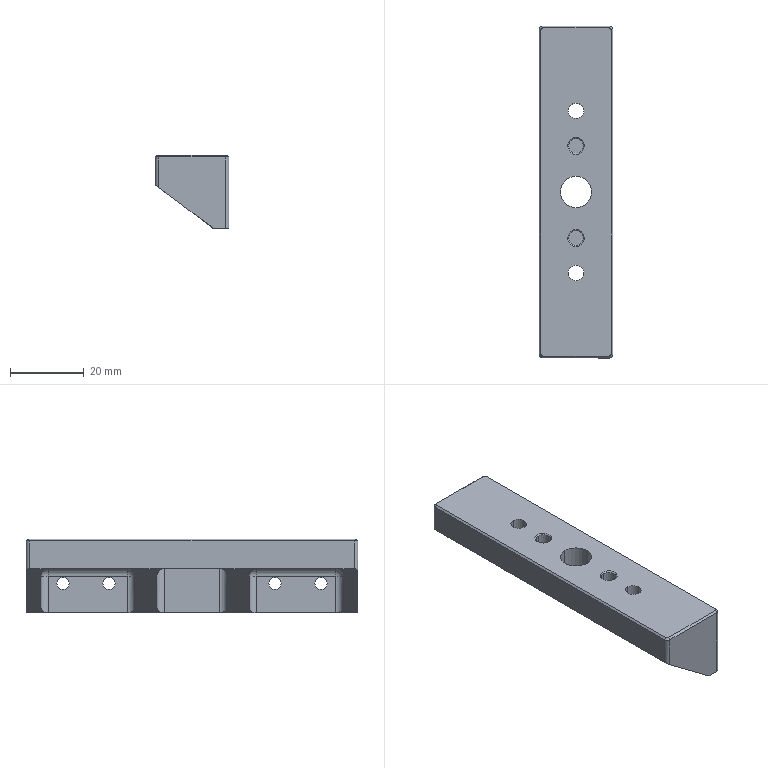NC program | NX | posted with a generic post | part box 20 x 90 x 20 mm
Lines 1 to 986 of 22268:
N10 G17 G21 G94 G90
(FLOOR_WALL_COPY , TOOL : D80)
N12 T19 M6
N14 G54
N16 G17 G0 G90 X-90. Y0. B0. C0. S6500 M3
N18 G43 Z30. H19
N20 Z7.
N22 G94 G1 Z4. F1500.
N24 X-85.
N26 X85.
N28 X90.
N30 Z7.
N32 G0 Z30.
N34 X-90.
N36 Z6.
N38 G1 Z3.
N40 X-85.
N42 X85.
N44 X90.
N46 Z6.
N48 G0 Z30.
N50 X-90.
N52 Z5.
N54 G1 Z2.
N56 X-85.
N58 X85.
N60 X90.
N62 Z5.
N64 G0 Z30.
N66 X-90.
N68 Z4.
N70 G1 Z1.
N72 X-85.
N74 X85.
N76 X90.
N78 Z4.
N80 G0 Z30.
N82 X-90.
N84 Z3.
N86 G1 Z0.
N88 X-85.
N90 X85.
N92 X90.
N94 Z3.
N96 G0 Z30.
N98 M5
(CAVITY_MILL , TOOL : D10)
N100 T15 M6
N102 G54
N104 G17 G0 G90 X-8.081 Y-16.996 B0. C0. S9500 M3
N106 G43 Z30. H15
N108 Z0.508
N110 G94 G1 Z-0.992 F1000.
N112 X-11.545 Y-10.996
N114 G3 X-12.411 Y-10.496 R1.
N116 G1 Y-5.996
N118 X-4.377 F3000.
N120 G2 X-2.441 Y-5.559 R4.5
N122 G1 X2.621 Y-5.56
N124 G2 X4.552 Y-5.996 R4.5
N126 G1 X20.578
N128 G2 X22.734 Y-5.541 R4.5
N130 G1 X23.214 Y-5.56
N132 X34.119
N134 G2 X36.052 Y-5.996 R4.5
N136 G1 X40.559
N138 Y-4.981
N140 G2 X35.921 Y-3.6 R9.806
N142 G1 X20.601
N144 G2 X15.634 Y-4.989 R10.196
N146 G1 X9.4
N148 G2 X4.42 Y-3.6 R9.73
N150 G1 X-4.431
N152 G2 X-9.404 Y-4.989 R9.73
N154 G1 X-15.645
N156 G2 X-20.601 Y-3.6 R10.226
N158 G1 X-35.924
N160 G2 X-40.559 Y-4.982 R9.72
N162 G1 Y-5.996
N164 X-35.876
N166 G2 X-33.941 Y-5.559 R4.5
N168 G1 X-22.377 Y-5.56
N170 G2 X-20.445 Y-5.996 R4.5
N172 G1 X-12.411
N174 Y-10.496
N176 X-2.465
N178 X-2.443 Y-10.184
N180 X-2.442 Y-10.059
N182 X2.619 Y-10.06
N184 G3 X2.654 Y-10.496 R5.476
N186 G1 X22.534
N188 X22.557 Y-10.038
N190 X23.126 Y-10.06
N192 X34.119
N194 G3 X34.154 Y-10.496 R5.269
N196 G1 X45.004
N198 X45.059 Y-10.493
N200 Y-0.488
N202 X40.909 Y-0.489
N204 G2 X37.372 Y0.9 R5.306
N206 G1 X19.19
N208 G2 X15.585 Y-0.489 R5.696
N210 G1 X9.409
N212 G2 X5.88 Y0.9 R5.23
N214 G1 X-5.891
N216 G2 X-9.415 Y-0.489 R5.23
N218 G1 X-15.591
N220 G2 X-19.193 Y0.9 R5.726
N222 G1 X-37.386
N224 G2 X-40.915 Y-0.489 R5.22
N226 G1 X-45.059 Y-0.488
N228 Y-1.888
N230 Y-10.493
N232 X-45.004 Y-10.496
N234 X-33.965
N236 X-33.943 Y-10.167
N238 X-33.941 Y-10.059
N240 X-22.378 Y-10.06
N242 X-22.345 Y-10.496
N244 X-12.411
N246 G2 X-11.545 Y-10.996 R1.
N248 G1 X-8.081 Y-16.996
N250 Z0.508
N252 G0 X-14.854 Z-0.483
N254 G1 Z-1.983 F1000.
N256 X-18.318 Y-10.996
N258 G3 X-19.184 Y-10.496 R1.
N260 G1 Y-5.996
N262 X-17.923 F3000.
N264 G2 X-22.174 Y-3.6 R9.614
N266 G1 X-34.345
N268 G2 X-38.549 Y-5.996 R9.442
N270 G1 X-35.876
N272 G2 X-33.941 Y-5.559 R4.5
N274 G1 X-22.377 Y-5.56
N276 G2 X-20.445 Y-5.996 R4.5
N278 G1 X-19.184
N280 Y-10.496
N282 X-7.071
N284 Y-5.996
N286 X-4.378
N288 G2 X-2.441 Y-5.559 R4.5
N290 G1 X2.621 Y-5.56
N292 G2 X4.552 Y-5.996 R4.5
N294 G1 X7.068
N296 G2 X2.827 Y-3.6 R9.58
N298 G1 X-2.828
N300 G2 X-7.071 Y-5.996 R9.584
N302 G1 Y-10.496
N304 X-2.465
N306 X-2.443 Y-10.184
N308 X-2.442 Y-10.059
N310 X2.619 Y-10.06
N312 G3 X2.654 Y-10.496 R5.476
N314 G1 X17.923
N316 Y-5.996
N318 X20.578
N320 G2 X22.734 Y-5.541 R4.5
N322 G1 X23.214 Y-5.56
N324 X34.119
N326 G2 X36.052 Y-5.996 R4.5
N328 G1 X38.549
N330 G2 X34.345 Y-3.6 R9.442
N332 G1 X22.174
N334 G2 X17.923 Y-5.996 R9.613
N336 G1 Y-10.496
N338 X22.534
N340 X22.557 Y-10.038
N342 X23.126 Y-10.06
N344 X34.119
N346 G3 X34.154 Y-10.496 R5.269
N348 G1 X45.004
N350 X45.059 Y-10.493
N352 Y-1.81
N354 X40.967 Y-1.811
N356 G2 X37.472 Y-0.363 R4.942
N358 X36.43 Y0.9 R8.564
N360 G1 X19.997
N362 G2 X15.5 Y-1.811 R5.113
N364 G1 X9.5
N366 G2 X5.011 Y0.9 R5.08
N368 G1 X-5.011
N370 G2 X-9.5 Y-1.811 R5.084
N372 G1 X-15.5
N374 G2 X-19.997 Y0.9 R5.114
N376 G1 X-36.43
N378 G2 X-37.472 Y-0.363 R8.564
N380 X-40.967 Y-1.811 R4.942
N382 G1 X-45.059 Y-1.81
N384 Y-3.211
N386 Y-10.493
N388 X-45.004 Y-10.496
N390 X-33.965
N392 X-33.943 Y-10.167
N394 X-33.941 Y-10.059
N396 X-22.378 Y-10.06
N398 X-22.345 Y-10.496
N400 X-19.184
N402 G2 X-18.318 Y-10.996 R1.
N404 G1 X-14.854 Y-16.996
N406 Z-0.483
N408 G0 X-17.797 Z-1.475
N410 G1 Z-2.975 F1000.
N412 X-21.512 Y-10.56
N414 G3 X-22.378 Y-10.06 R1.
N416 G1 X-22.377 Y-5.56
N418 G2 X-21.26 Y-5.701 R4.5 F3000.
N420 X-23.306 Y-3.6 R9.607
N422 G1 X-33.193
N424 G2 X-35.355 Y-5.787 R9.605
N426 X-33.941 Y-5.559 R4.5
N428 G1 X-22.377 Y-5.56
N430 X-22.378 Y-10.06
N432 X-22.345 Y-10.496
N434 X-2.465
N436 X-2.443 Y-10.184
N438 X-2.442 Y-10.059
N440 X-3.852 Y-5.785
N442 G2 X-2.441 Y-5.559 R4.5
N444 G1 X2.621 Y-5.56
N446 G2 X3.74 Y-5.702 R4.5
N448 X1.693 Y-3.6 R9.606
N450 G1 X-1.693
N452 G2 X-3.852 Y-5.785 R9.602
N454 G1 X-2.442 Y-10.059
N456 X2.619 Y-10.06
N458 G3 X2.654 Y-10.496 R5.476
N460 G1 X22.534
N462 X22.557 Y-10.038
N464 X21.195 Y-5.749
N466 G2 X22.734 Y-5.541 R4.5
N468 G1 X23.214 Y-5.56
N470 X34.119
N472 G2 X35.24 Y-5.702 R4.5
N474 X33.194 Y-3.6 R9.602
N476 G1 X23.305
N478 G2 X21.195 Y-5.749 R9.608
N480 G1 X22.557 Y-10.038
N482 X23.126 Y-10.06
N484 X34.119
N486 G3 X34.154 Y-10.496 R5.269
N488 G1 X45.004
N490 X45.059 Y-10.493
N492 Y-3.133
N494 X41.
N496 G2 X36.027 Y0.9 R5.102
N498 G1 X20.474
N500 G2 X15.5 Y-3.133 R5.108
N502 G1 X9.5
N504 G2 X4.525 Y0.9 R5.106
N506 G1 X-4.527
N508 G2 X-9.5 Y-3.133 R5.102
N510 G1 X-15.5
N512 G2 X-20.474 Y0.9 R5.107
N514 G1 X-36.026
N516 G2 X-41. Y-3.133 R5.105
N518 G1 X-45.059
N520 Y-10.493
N522 X-45.004 Y-10.496
N524 X-33.965
N526 X-33.943 Y-10.167
N528 X-33.941 Y-10.059
N530 X-22.378 Y-10.06
N532 G2 X-21.512 Y-10.56 R1.
N534 G1 X-17.797 Y-16.996
N536 Z-1.475
N538 G0 X-23.669 Y-16.997 Z-2.467
N540 G1 Z-3.967 F1000.
N542 X-27.384 Y-10.56
N544 G3 X-28.25 Y-10.06 R1.
N546 G1 Y-5.56
N548 X-22.808 F3000.
N550 G2 X-24.098 Y-3.6 R9.633
N552 G1 X-32.402
N554 G2 X-33.692 Y-5.559 R9.635
N556 G1 X-28.25 Y-5.56
N558 Y-10.06
N560 X-22.378
N562 X-22.345 Y-10.497
N564 X-2.465
N566 X-2.443 Y-10.184
N568 X-2.442 Y-10.059
N570 X-2.21
N572 X-2.208 Y-5.559
N574 X2.209 Y-5.56
N576 G2 X0.914 Y-3.6 R9.666
N578 G1 X-0.914
N580 G2 X-2.208 Y-5.559 R9.666
N582 G1 X-2.21 Y-10.059
N584 X2.619 Y-10.06
N586 G3 X2.654 Y-10.497 R5.476
N588 G1 X22.534
N590 X22.557 Y-10.038
N592 X22.644 Y-10.041
N594 X22.821 Y-5.545
N596 X23.214 Y-5.56
N598 X33.693
N600 G2 X32.402 Y-3.6 R9.635
N602 G1 X24.098
N604 G2 X22.821 Y-5.545 R9.634
N606 G1 X22.644 Y-10.041
N608 X23.126 Y-10.06
N610 X34.119
N612 G3 X34.154 Y-10.497 R5.269
N614 G1 X45.003
N616 X45.059 Y-10.493
N618 Y-4.455
N620 X41. Y-4.456
N622 G2 X35.904 Y0.475 R5.135
N624 X35.9 Y0.782 R5.136
N626 G1 X35.904 Y0.9
N628 X20.6
N630 Y0.712
N632 G2 X15.5 Y-4.456 R5.134
N634 G1 X9.476 Y-4.455
N636 G2 X4.508 Y-0.339 R5.166
N638 X4.4 Y0.756 R5.166
N640 G1 X4.401 Y0.9
N642 X-4.4
N644 Y0.711
N646 G2 X-9.5 Y-4.456 R5.166
N648 G1 X-15.5
N650 G2 X-20.546 Y-0.068 R5.133
N652 X-20.6 Y0.746 R5.134
N654 G1 X-20.597 Y0.9
N656 X-35.9
N658 Y0.711
N660 G2 X-41. Y-4.456 R5.135
N662 G1 X-45.059 Y-4.455
N664 Y-10.493
N666 X-45.003 Y-10.497
N668 X-33.965
N670 X-33.943 Y-10.167
N672 X-33.941 Y-10.059
N674 X-28.25 Y-10.06
N676 G2 X-27.384 Y-10.56 R1.
N678 G1 X-23.669 Y-16.997
N680 Z-2.467
N682 G0 X-23.671 Z-3.458
N684 G1 Z-4.958 F1000.
N686 X-27.387 Y-10.56
N688 G3 X-28.253 Y-10.06 R1.
N690 G1 Y-5.56
N692 X-23.752 F3000.
N694 G2 X-24.636 Y-3.6 R9.633
N696 G1 X-31.868
N698 G2 X-32.754 Y-5.559 R9.647
N700 G1 X-28.253 Y-5.56
N702 Y-10.06
N704 X-22.378
N706 X-22.345 Y-10.497
N708 X-2.465
N710 X-2.443 Y-10.184
N712 X-2.442 Y-10.059
N714 X-1.268
N716 X-1.267 Y-5.559
N718 X1.267 Y-5.56
N720 G2 X0.377 Y-3.6 R9.678
N722 G1 X-0.377
N724 G2 X-1.267 Y-5.559 R9.678
N726 G1 X-1.268 Y-10.059
N728 X2.619 Y-10.06
N730 G3 X2.654 Y-10.497 R5.476
N732 G1 X22.534
N734 X22.557 Y-10.038
N736 X23.126 Y-10.06
N738 X23.752
N740 Y-5.56
N742 X32.754
N744 G2 X31.868 Y-3.6 R9.647
N746 G1 X24.636
N748 G2 X23.752 Y-5.56 R9.633
N750 G1 Y-10.06
N752 X34.119
N754 G3 X34.154 Y-10.497 R5.269
N756 G1 X45.003
N758 X45.059 Y-10.494
N760 Y-5.777
N762 X41. Y-5.778
N764 G2 X35.9 Y-0.611 R5.147
N766 G1 Y-0.5
N768 Y0.782
N770 X35.903 Y0.9
N772 X20.6
N774 Y-0.611
N776 G2 X15.5 Y-5.778 R5.133
N778 G1 X9.5
N780 G2 X4.4 Y-0.611 R5.178
N782 G1 Y0.9
N784 X-4.4
N786 Y-0.611
N788 G2 X-9.5 Y-5.778 R5.178
N790 G1 X-15.5
N792 G2 X-20.6 Y-0.611 R5.133
N794 G1 Y0.746
N796 X-20.597 Y0.9
N798 X-35.9
N800 Y-0.611
N802 G2 X-41. Y-5.778 R5.147
N804 G1 X-45.059 Y-5.777
N806 Y-10.494
N808 X-45.003 Y-10.497
N810 X-33.965
N812 X-33.943 Y-10.167
N814 X-33.941 Y-10.059
N816 X-28.253 Y-10.06
N818 G2 X-27.387 Y-10.56 R1.
N820 G1 X-23.671 Y-16.997
N822 Z-3.458
N824 G0 X-23.668 Z-4.45
N826 G1 Z-5.95 F1000.
N828 X-27.384 Y-10.56
N830 G3 X-28.25 Y-10.06 R1.
N832 G1 Y-5.56
N834 X-24.405 F3000.
N836 G2 X-24.961 Y-3.6 R9.633
N838 G1 X-31.539
N840 G2 X-32.095 Y-5.559 R9.633
N842 G1 X-28.25 Y-5.56
N844 Y-10.06
N846 X-22.378
N848 X-22.345 Y-10.497
N850 X-2.465
N852 X-2.443 Y-10.184
N854 X-2.442 Y-10.059
N856 X-0.596
N858 X-0.595 Y-5.559
N860 X0.595
N862 G2 X0.039 Y-3.6 R9.633
N864 G1 X-0.039
N866 G2 X-0.595 Y-5.559 R9.633
N868 G1 X-0.596 Y-10.059
N870 X2.619 Y-10.06
N872 G3 X2.654 Y-10.497 R5.476
N874 G1 X22.534
N876 X22.557 Y-10.038
N878 X23.126 Y-10.06
N880 X24.405
N882 Y-5.56
N884 X32.095
N886 G2 X31.539 Y-3.6 R9.633
N888 G1 X24.961
N890 G2 X24.405 Y-5.56 R9.633
N892 G1 Y-10.06
N894 X34.119
N896 G3 X34.154 Y-10.497 R5.269
N898 G1 X45.003
N900 X45.059 Y-10.494
N902 Y-7.099
N904 X41. Y-7.1
N906 G2 X35.9 Y-1.933 R5.133
N908 G1 Y0.782
N910 X35.903 Y0.9
N912 X20.6
N914 Y-1.933
N916 G2 X15.5 Y-7.1 R5.133
N918 G1 X9.475
N920 G2 X4.4 Y-1.933 R5.133
N922 G1 Y0.9
N924 X-4.4
N926 Y-1.933
N928 G2 X-9.5 Y-7.1 R5.133
N930 G1 X-15.5
N932 G2 X-20.6 Y-1.933 R5.133
N934 G1 Y0.746
N936 X-20.598 Y0.9
N938 X-35.9
N940 Y-1.933
N942 G2 X-41. Y-7.1 R5.133
N944 G1 X-45.059 Y-7.099
N946 Y-10.494
N948 X-45.003 Y-10.497
N950 X-33.965
N952 X-33.943 Y-10.167
N954 X-33.941 Y-10.059
N956 X-28.25 Y-10.06
N958 G2 X-27.384 Y-10.56 R1.
N960 G1 X-23.668 Y-16.997
N962 Z-4.45
N964 G0 Z-5.442
N966 G1 Z-6.942 F1000.
N968 X-27.384 Y-10.56
N970 G3 X-28.25 Y-10.06 R1.
N972 G1 Y-5.56
N974 X-24.829 F3000.
N976 G2 X-25.095 Y-3.6 R9.633
N978 G1 X-31.405
N980 G2 X-31.671 Y-5.559 R9.633
N982 G1 X-28.25 Y-5.56
N984 Y-10.06
N986 X-22.378
N988 X-22.345 Y-10.497
N990 X-2.465
N992 X-2.443 Y-10.184
N994 X-2.442 Y-10.059
N996 X-0.172
N998 X-0.171 Y-5.559
N1000 X0.171
N1002 G2 X0. Y-4.674 R9.633
N1004 X-0.171 Y-5.559 R9.633
N1006 G1 X-0.172 Y-10.059
N1008 X2.619 Y-10.06
N1010 G3 X2.654 Y-10.497 R5.476
N1012 G1 X22.534
N1014 X22.557 Y-10.038
N1016 X23.126 Y-10.06
N1018 X24.829
N1020 Y-5.56
N1022 X31.671
N1024 G2 X31.405 Y-3.6 R9.633
N1026 G1 X25.095
N1028 G2 X24.829 Y-5.56 R9.633
N1030 G1 Y-10.06
N1032 X34.119
N1034 G3 X34.154 Y-10.497 R5.269
N1036 G1 X45.003
N1038 X45.059 Y-10.494
N1040 Y-8.421
N1042 X41. Y-8.422
N1044 G2 X35.9 Y-3.256 R5.133
N1046 G1 Y0.782
N1048 X35.902 Y0.9
N1050 X20.6
N1052 Y-3.256
N1054 G2 X15.5 Y-8.422 R5.133
N1056 G1 X9.5
N1058 G2 X4.4 Y-3.256 R5.133
N1060 G1 Y0.9
N1062 X-4.4
N1064 Y-3.256
N1066 G2 X-9.5 Y-8.422 R5.133
N1068 G1 X-15.5
N1070 G2 X-20.6 Y-3.256 R5.133
N1072 G1 Y0.746
N1074 X-20.598 Y0.9
N1076 X-35.9
N1078 Y-3.256
N1080 G2 X-41. Y-8.422 R5.133
N1082 G1 X-45.059 Y-8.421
N1084 Y-10.494
N1086 X-45.003 Y-10.497
N1088 X-33.965
N1090 X-33.943 Y-10.167
N1092 X-33.941 Y-10.059
N1094 X-28.25 Y-10.06
N1096 G2 X-27.384 Y-10.56 R1.
N1098 G1 X-23.668 Y-16.997
N1100 Z-5.442
N1102 G0 Z-6.433
N1104 G1 Z-7.933 F1000.
N1106 X-27.385 Y-10.56
N1108 G3 X-28.251 Y-10.06 R1.
N1110 G1 X-28.25 Y-5.56
N1112 X-25.053 F3000.
N1114 G2 X-25.1 Y-4.567 R9.639
N1116 G1 Y-3.6
N1118 X-31.4
N1120 Y-4.569
N1122 G2 X-31.448 Y-5.559 R9.643
N1124 G1 X-28.25 Y-5.56
N1126 X-28.251 Y-10.06
N1128 X-22.378
N1130 X-22.345 Y-10.497
N1132 X-18.298
N1134 G3 X-15.5 Y-11.144 R6.539
N1136 G1 X-9.478
N1138 G3 X-6.733 Y-10.497 R6.58
N1140 G1 X-2.465
N1142 X-2.443 Y-10.184
N1144 X-2.442 Y-10.059
N1146 X2.619 Y-10.06
N1148 G3 X2.654 Y-10.497 R5.476
N1150 G1 X6.733
N1152 G3 X9.5 Y-11.144 R6.58
N1154 G1 X15.511
N1156 G3 X18.298 Y-10.497 R6.539
N1158 G1 X22.534
N1160 X22.557 Y-10.038
N1162 X23.126 Y-10.06
N1164 X25.053
N1166 Y-5.56
N1168 X31.448
N1170 G2 X31.4 Y-4.569 R9.643
N1172 G1 Y-3.6
N1174 X25.1
N1176 Y-4.567
N1178 G2 X25.053 Y-5.56 R9.639
N1180 G1 Y-10.06
N1182 X34.119
N1184 G3 X34.154 Y-10.497 R5.269
N1186 G1 X38.205
N1188 G3 X41. Y-11.144 R6.543
N1190 G1 X45.059
N1192 Y-9.743
N1194 X41. Y-9.744
N1196 G2 X35.9 Y-4.578 R5.143
N1198 G1 Y0.782
N1200 X35.901 Y0.9
N1202 X20.6
N1204 Y-4.578
N1206 G2 X15.5 Y-9.744 R5.139
N1208 G1 X9.5
N1210 G2 X4.4 Y-4.578 R5.18
N1212 G1 Y0.9
N1214 X-4.4
N1216 Y-4.578
N1218 G2 X-9.5 Y-9.744 R5.18
N1220 G1 X-15.529
N1222 G2 X-20.6 Y-4.578 R5.139
N1224 G1 Y0.746
N1226 X-20.599 Y0.9
N1228 X-35.9
N1230 Y-4.578
N1232 G2 X-41. Y-9.744 R5.143
N1234 G1 X-45.059 Y-9.743
N1236 Y-10.494
N1238 Y-11.144
N1240 X-40.988
N1242 G3 X-38.205 Y-10.497 R6.543
N1244 G1 X-33.965
N1246 X-33.943 Y-10.167
N1248 X-33.941 Y-10.059
N1250 X-28.251 Y-10.06
N1252 G2 X-27.385 Y-10.56 R1.
N1254 G1 X-23.668 Y-16.997
N1256 Z-6.433
N1258 G0 Z-7.425
N1260 G1 Z-8.925 F1000.
N1262 X-27.384 Y-10.56
N1264 G3 X-28.25 Y-10.06 R1.
N1266 G1 Y-5.56
N1268 X-25.1 F3000.
N1270 Y-3.6
N1272 X-31.4
N1274 Y-5.559
N1276 X-28.25 Y-5.56
N1278 Y-10.06
N1280 X-22.378
N1282 X-22.345 Y-10.497
N1284 X-20.142
N1286 G3 X-15.5 Y-12.467 R6.533
N1288 G1 X-9.482
N1290 G3 X-4.878 Y-10.497 R6.567
N1292 G1 X-2.465
N1294 X-2.443 Y-10.184
N1296 X-2.442 Y-10.059
N1298 X2.619 Y-10.06
N1300 G3 X2.654 Y-10.497 R5.476
N1302 G1 X4.878
N1304 G3 X9.5 Y-12.467 R6.567
N1306 G1 X15.509
N1308 G3 X20.142 Y-10.497 R6.533
N1310 G1 X22.534
N1312 X22.557 Y-10.038
N1314 X23.126 Y-10.06
N1316 X25.1
N1318 Y-5.56
N1320 X31.4
N1322 Y-3.6
N1324 X25.1
N1326 Y-5.56
N1328 Y-10.06
N1330 X34.119
N1332 G3 X34.154 Y-10.497 R5.269
N1334 G1 X36.365
N1336 G3 X41. Y-12.467 R6.544
N1338 G1 X45.059 Y-12.466
N1340 Y-11.066
N1342 X41. Y-11.067
N1344 G2 X35.9 Y-5.9 R5.144
N1346 G1 Y0.782
N1348 X35.901 Y0.9
N1350 X34.501
N1352 X20.6
N1354 Y-5.9
N1356 G2 X15.5 Y-11.067 R5.133
N1358 G1 X9.5
N1360 G2 X4.4 Y-5.9 R5.167
N1362 G1 Y0.9
N1364 X-4.4
N1366 Y-5.9
N1368 G2 X-9.5 Y-11.067 R5.167
N1370 G1 X-15.5
N1372 G2 X-20.6 Y-5.9 R5.133
N1374 G1 Y0.746
N1376 X-20.599 Y0.9
N1378 X-21.999
N1380 X-35.9
N1382 Y-5.9
N1384 G2 X-41. Y-11.067 R5.144
N1386 G1 X-45.059 Y-11.066
N1388 Y-12.466
N1390 X-40.988 Y-12.467
N1392 G3 X-36.365 Y-10.497 R6.544
N1394 G1 X-33.965
N1396 X-33.943 Y-10.167
N1398 X-33.941 Y-10.059
N1400 X-28.25 Y-10.06
N1402 G2 X-27.384 Y-10.56 R1.
N1404 G1 X-23.668 Y-16.997
N1406 Z-7.425
N1408 G0 Y-16.998 Z-8.417
N1410 G1 Z-9.917 F1000.
N1412 X-27.384 Y-10.56
N1414 G3 X-28.25 Y-10.06 R1.
N1416 G1 Y-5.56
N1418 X-25.1 F3000.
N1420 Y-3.6
N1422 X-31.4
N1424 Y-5.559
N1426 X-28.25 Y-5.56
N1428 Y-10.06
N1430 X-22.378
N1432 X-22.345 Y-10.498
N1434 X-21.134
N1436 G3 X-15.5 Y-13.789 R6.545
N1438 G1 X-9.491
N1440 G3 X-3.861 Y-10.498 R6.533
N1442 G1 X-2.465
N1444 X-2.443 Y-10.184
N1446 X-2.442 Y-10.059
N1448 X2.619 Y-10.06
N1450 G3 X2.654 Y-10.498 R5.476
N1452 G1 X3.862
N1454 G3 X9.5 Y-13.789 R6.535
N1456 G1 X15.509
N1458 G3 X21.139 Y-10.498 R6.533
N1460 G1 X22.534
N1462 X22.557 Y-10.038
N1464 X23.126 Y-10.06
N1466 X25.1
N1468 Y-5.56
N1470 X31.4
N1472 Y-3.6
N1474 X25.1
N1476 Y-5.56
N1478 Y-10.06
N1480 X34.119
N1482 G3 X34.154 Y-10.498 R5.269
N1484 G1 X35.361
N1486 G3 X41. Y-13.789 R6.533
N1488 G1 X45.045
N1490 X45.059 Y-13.586
N1492 Y-12.388
N1494 X41. Y-12.389
N1496 G2 X35.9 Y-7.222 R5.133
N1498 G1 Y-5.56
N1500 Y0.9
N1502 X20.6
N1504 Y-7.222
N1506 G2 X15.5 Y-12.389 R5.133
N1508 G1 X9.474
N1510 G2 X4.4 Y-7.222 R5.135
N1512 G1 Y0.9
N1514 X-4.4
N1516 Y-7.222
N1518 G2 X-9.5 Y-12.389 R5.133
N1520 G1 X-15.5
N1522 G2 X-20.6 Y-7.222 R5.145
N1524 G1 Y0.746
N1526 Y0.9
N1528 X-35.9
N1530 Y-7.222
N1532 G2 X-41. Y-12.389 R5.133
N1534 G1 X-45.059 Y-12.388
N1536 Y-13.585
N1538 X-45.062 Y-13.788
N1540 X-40.991 Y-13.789
N1542 G3 X-35.361 Y-10.498 R6.533
N1544 G1 X-33.965
N1546 X-33.943 Y-10.167
N1548 X-33.941 Y-10.059
N1550 X-28.25 Y-10.06
N1552 G2 X-27.384 Y-10.56 R1.
N1554 G1 X-23.668 Y-16.998
N1556 Z-8.417
N1558 G0 Z-9.408
N1560 G1 Z-10.908 F1000.
N1562 X-27.384 Y-10.56
N1564 G3 X-28.25 Y-10.06 R1.
N1566 G1 Y-5.56
N1568 X-25.331 F3000.
N1570 Y-3.831
N1572 X-31.169
N1574 Y-5.559
N1576 X-28.25 Y-5.56
N1578 Y-10.06
N1580 X-22.378
N1582 X-22.345 Y-10.498
N1584 X-21.962
N1586 G3 X-16.978 Y-14.998 R6.458
N1588 G1 X-8.048
N1590 G3 X-3.045 Y-10.498 R6.487
N1592 G1 X-2.465
N1594 X-2.443 Y-10.184
N1596 X-2.442 Y-10.059
N1598 X2.619 Y-10.06
N1600 G3 X2.654 Y-10.498 R5.476
N1602 G1 X3.045
N1604 G3 X8.048 Y-14.998 R6.486
N1606 G1 X16.952
N1608 G3 X21.955 Y-10.498 R6.487
N1610 G1 X22.534
N1612 X22.557 Y-10.038
N1614 X23.126 Y-10.06
N1616 X25.331
N1618 Y-5.56
N1620 X31.169
N1622 Y-3.831
N1624 X25.331
N1626 Y-5.56
N1628 Y-10.06
N1630 X34.119
N1632 G3 X34.154 Y-10.498 R5.269
N1634 G1 X34.545
N1636 G3 X39.548 Y-14.998 R6.486
N1638 G1 X44.492
N1640 X44.603 Y-14.929
N1642 X44.748 Y-14.809
N1644 X44.976 Y-14.635
N1646 X45.019 Y-14.628
N1648 X44.999 Y-14.589
N1650 X45.006 Y-14.355
N1652 X45.051 Y-13.71
N1654 X40.735 Y-13.711
N1656 G2 X35.669 Y-8.605 R5.086
N1658 G1 Y-0.731
N1660 Y0.669
N1662 X20.831
N1664 Y-0.731
N1666 Y-8.606
N1668 G2 X15.761 Y-13.711 R5.087
N1670 G1 X9.235
N1672 G2 X4.169 Y-8.605 R5.086
N1674 G1 Y0.9
N1676 X-4.169
N1678 Y-8.606
N1680 G2 X-9.239 Y-13.711 R5.087
N1682 G1 X-15.773
N1684 G2 X-20.831 Y-8.653 R5.058
N1686 G1 Y-0.731
N1688 Y0.669
N1690 X-35.669
N1692 Y-0.731
N1694 Y-8.606
N1696 G2 X-40.739 Y-13.711 R5.087
N1698 G1 X-45.061 Y-13.71
N1700 X-45.068 Y-14.251
N1702 X-45.061 Y-14.28
N1704 X-45.007 Y-14.378
N1706 X-44.903 Y-14.606
N1708 X-44.699 Y-14.88
N1710 X-44.674 Y-14.9
N1712 X-44.442 Y-14.998
N1714 X-39.548
N1716 G3 X-34.545 Y-10.498 R6.487
N1718 G1 X-33.965
N1720 X-33.943 Y-10.167
N1722 X-33.941 Y-10.059
N1724 X-28.25 Y-10.06
N1726 G2 X-27.384 Y-10.56 R1.
N1728 G1 X-23.668 Y-16.998
N1730 Z-9.408
N1732 G0 Z-10.4
N1734 G1 Z-11.9 F1000.
N1736 X-27.384 Y-10.56
N1738 G3 X-28.25 Y-10.06 R1.
N1740 G1 Y-5.56
N1742 X-26.831 F3000.
N1744 Y-5.331
N1746 X-29.669
N1748 Y-5.559
N1750 X-28.25 Y-5.56
N1752 Y-10.06
N1754 X-22.378
N1756 X-22.341 Y-10.534
N1758 X-22.196 Y-11.309
N1760 X-21.916 Y-12.086
N1762 X-21.785 Y-12.293
N1764 X-21.701 Y-12.507
N1766 X-21.692 Y-12.563
N1768 X-21.637 Y-12.547
N1770 X-21.613 Y-12.584
N1772 X-21.606 Y-12.656
N1774 X-21.597 Y-12.682
N1776 X-21.53 Y-12.781
N1778 X-21.433 Y-12.862
N1780 X-20.853 Y-13.609
N1782 X-20.242 Y-14.14
N1784 X-20.181 Y-14.167
N1786 G3 X-18.232 Y-14.998 R5.26
N1788 G1 X-17.638
N1790 G2 X-22.331 Y-9.757 R5.211
N1792 G1 Y-0.831
N1794 X-34.169
N1796 Y-9.989
N1798 G2 X-38.753 Y-14.998 R5.096
N1800 G1 X-38.265
N1802 G3 X-36.557 Y-14.403 R6.548
N1804 X-34.111 Y-11.299 R5.676
N1806 G1 X-33.967 Y-10.527
N1808 X-33.965 Y-10.498
N1810 X-33.942 Y-10.131
N1812 X-33.941 Y-10.059
N1814 X-28.25 Y-10.06
N1816 G2 X-27.384 Y-10.56 R1.
N1818 G1 X-23.668 Y-16.998
N1820 Z-10.4
N1822 G0 Z30.
N1824 X-4.497
N1826 Z-10.4
N1828 G1 Z-11.9 F1000.
N1830 X-0.777 Y-10.559
N1832 G2 X0.089 Y-10.059 R1.
N1834 G1 X2.619 Y-10.06 F3000.
N1836 G3 X2.654 Y-10.498 R5.476
N1838 X3.513 Y-12.851 R5.476
N1840 G1 X3.801 Y-13.394
N1842 X3.823 Y-13.417
N1844 X4.172 Y-13.634
N1846 X4.547 Y-13.963
N1848 X4.593 Y-13.988
N1850 G3 X6.838 Y-14.998 R5.931
N1852 G1 X7.362
N1854 G2 X2.669 Y-9.757 R5.211
N1856 G1 Y0.9
N1858 X-2.669
N1860 Y-9.757
N1862 G2 X-7.364 Y-14.998 R5.213
N1864 G1 X-6.806
N1866 G3 X-5.057 Y-14.403 R7.153
N1868 X-2.61 Y-11.299 R5.701
N1870 G1 X-2.467 Y-10.527
N1872 X-2.443 Y-10.184
N1874 X-2.442 Y-10.059
N1876 X0.089
N1878 G2 X0.955 Y-10.56 R1.
N1880 G1 X4.669 Y-16.998
N1882 Z-10.4
N1884 G0 Z30.
N1886 X32.833
N1888 Z-10.4
N1890 G1 Z-11.9 F1000.
N1892 X29.116 Y-10.56
N1894 G3 X28.25 Y-10.06 R1.
N1896 G1 Y-5.56
N1898 X29.669 F3000.
N1900 Y-5.331
N1902 X26.831
N1904 Y-5.56
N1906 X28.25
N1908 Y-10.06
N1910 X34.119
N1912 G3 X35.224 Y-13.096 R5.269
N1914 X36.755 Y-14.404 R3.934
N1916 G1 X36.98 Y-14.556
N1918 X37.76 Y-14.868
N1920 X38.322 Y-14.998
N1922 X38.862
N1924 G2 X34.169 Y-9.757 R5.211
N1926 G1 Y-0.831
N1928 X22.331
N1930 Y-9.989
N1932 G2 X17.747 Y-14.998 R5.096
N1934 G1 X18.304
N1936 G3 X20.962 Y-13.625 R5.292
N1938 G1 X21.946 Y-12.493
N1940 X21.957 Y-12.474
N1942 X22.388 Y-11.304
N1944 X22.415 Y-11.201
N1946 X22.533 Y-10.525
N1948 X22.534 Y-10.498
N1950 X22.557 Y-10.038
N1952 X23.126 Y-10.06
N1954 X28.25
N1956 G2 X29.116 Y-10.56 R1.
N1958 G1 X32.833 Y-16.998
N1960 Z-10.4
N1962 G0 Z30.
N1964 M5